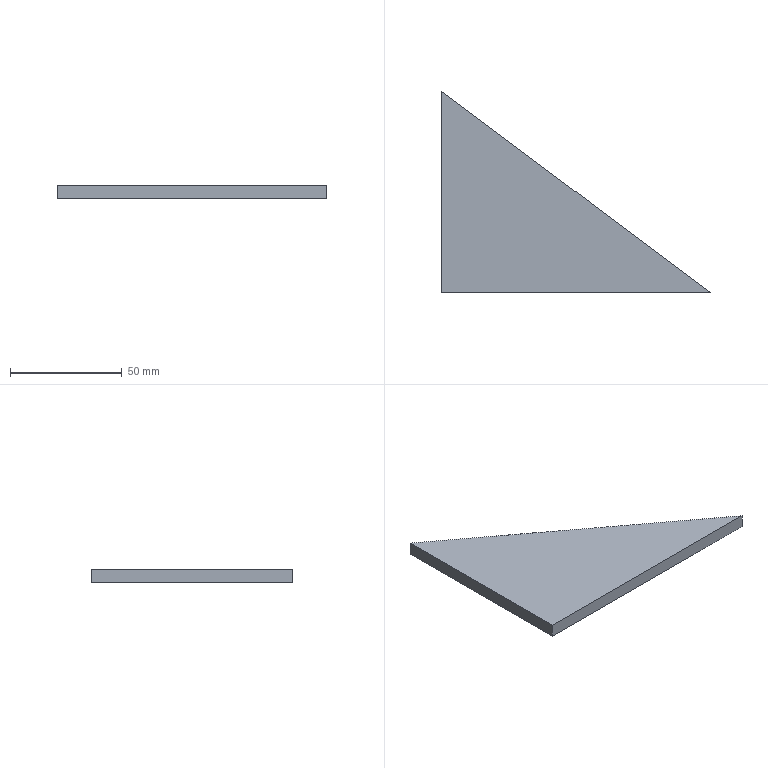Part | STEP file | BCC3 H17_3 | 1 solid | 5 faces | box 120 x 90 x 6 mm | volume 32400 mm3 | plane 5
STEP:
#1=CARTESIAN_POINT('',(0.,0.,0.));
#2=DIRECTION('',(0.,0.,1.));
#3=DIRECTION('',(1.,0.,0.));
#4=AXIS2_PLACEMENT_3D('',#1,#2,#3);
#5=CARTESIAN_POINT('',(0.,0.,0.));
#6=VERTEX_POINT('',#5);
#7=CARTESIAN_POINT('',(120.,0.,0.));
#8=VERTEX_POINT('',#7);
#9=CARTESIAN_POINT('',(120.,0.,0.));
#10=DIRECTION('',(1.,0.,0.));
#11=VECTOR('',#10,1.);
#12=LINE('',#9,#11);
#13=CARTESIAN_POINT('',(120.,0.,6.));
#14=DIRECTION('',(0.,1.,0.));
#15=DIRECTION('',(-1.,0.,0.));
#16=AXIS2_PLACEMENT_3D('',#13,#14,#15);
#17=PLANE('',#16);
#18=CARTESIAN_POINT('',(0.,-6.));
#19=DIRECTION('',(-1.,0.));
#20=VECTOR('',#19,1.);
#21=LINE('',#18,#20);
#22=(GEOMETRIC_REPRESENTATION_CONTEXT(2)PARAMETRIC_REPRESENTATION_CONTEXT()REPRESENTATION_CONTEXT('',''));
#23=DEFINITIONAL_REPRESENTATION('',(#21),#22);
#24=PCURVE('',#17,#23);
#25=CARTESIAN_POINT('',(0.,0.,0.));
#26=DIRECTION('',(0.,0.,-1.));
#27=DIRECTION('',(-1.,0.,0.));
#28=AXIS2_PLACEMENT_3D('',#25,#26,#27);
#29=PLANE('',#28);
#30=CARTESIAN_POINT('',(-120.,0.));
#31=DIRECTION('',(-1.,0.));
#32=VECTOR('',#31,1.);
#33=LINE('',#30,#32);
#34=(GEOMETRIC_REPRESENTATION_CONTEXT(2)PARAMETRIC_REPRESENTATION_CONTEXT()REPRESENTATION_CONTEXT('',''));
#35=DEFINITIONAL_REPRESENTATION('',(#33),#34);
#36=PCURVE('',#29,#35);
#37=SURFACE_CURVE('',#12,(#24,#36),.PCURVE_S1.);
#38=EDGE_CURVE('',#6,#8,#37,.T.);
#39=ORIENTED_EDGE('',*,*,#38,.T.);
#40=CARTESIAN_POINT('',(120.,0.,6.));
#41=VERTEX_POINT('',#40);
#42=CARTESIAN_POINT('',(120.,0.,6.));
#43=DIRECTION('',(0.,0.,-1.));
#44=VECTOR('',#43,1.);
#45=LINE('',#42,#44);
#46=CARTESIAN_POINT('',(0.,0.));
#47=DIRECTION('',(0.,-1.));
#48=VECTOR('',#47,1.);
#49=LINE('',#46,#48);
#50=(GEOMETRIC_REPRESENTATION_CONTEXT(2)PARAMETRIC_REPRESENTATION_CONTEXT()REPRESENTATION_CONTEXT('',''));
#51=DEFINITIONAL_REPRESENTATION('',(#49),#50);
#52=PCURVE('',#17,#51);
#53=CARTESIAN_POINT('',(0.,90.,6.));
#54=DIRECTION('',(-0.6,-0.8,0.));
#55=DIRECTION('',(0.8,-0.6,0.));
#56=AXIS2_PLACEMENT_3D('',#53,#54,#55);
#57=PLANE('',#56);
#58=CARTESIAN_POINT('',(150.,0.));
#59=DIRECTION('',(0.,-1.));
#60=VECTOR('',#59,1.);
#61=LINE('',#58,#60);
#62=(GEOMETRIC_REPRESENTATION_CONTEXT(2)PARAMETRIC_REPRESENTATION_CONTEXT()REPRESENTATION_CONTEXT('',''));
#63=DEFINITIONAL_REPRESENTATION('',(#61),#62);
#64=PCURVE('',#57,#63);
#65=SURFACE_CURVE('',#45,(#52,#64),.PCURVE_S1.);
#66=EDGE_CURVE('',#41,#8,#65,.T.);
#67=ORIENTED_EDGE('',*,*,#66,.F.);
#68=CARTESIAN_POINT('',(0.,0.,6.));
#69=VERTEX_POINT('',#68);
#70=CARTESIAN_POINT('',(120.,0.,6.));
#71=DIRECTION('',(1.,0.,0.));
#72=VECTOR('',#71,1.);
#73=LINE('',#70,#72);
#74=CARTESIAN_POINT('',(0.,0.));
#75=DIRECTION('',(-1.,0.));
#76=VECTOR('',#75,1.);
#77=LINE('',#74,#76);
#78=(GEOMETRIC_REPRESENTATION_CONTEXT(2)PARAMETRIC_REPRESENTATION_CONTEXT()REPRESENTATION_CONTEXT('',''));
#79=DEFINITIONAL_REPRESENTATION('',(#77),#78);
#80=PCURVE('',#17,#79);
#81=CARTESIAN_POINT('',(0.,0.,6.));
#82=DIRECTION('',(0.,0.,-1.));
#83=DIRECTION('',(-1.,0.,0.));
#84=AXIS2_PLACEMENT_3D('',#81,#82,#83);
#85=PLANE('',#84);
#86=CARTESIAN_POINT('',(-120.,0.));
#87=DIRECTION('',(-1.,0.));
#88=VECTOR('',#87,1.);
#89=LINE('',#86,#88);
#90=(GEOMETRIC_REPRESENTATION_CONTEXT(2)PARAMETRIC_REPRESENTATION_CONTEXT()REPRESENTATION_CONTEXT('',''));
#91=DEFINITIONAL_REPRESENTATION('',(#89),#90);
#92=PCURVE('',#85,#91);
#93=SURFACE_CURVE('',#73,(#80,#92),.PCURVE_S1.);
#94=EDGE_CURVE('',#69,#41,#93,.T.);
#95=ORIENTED_EDGE('',*,*,#94,.F.);
#96=CARTESIAN_POINT('',(0.,0.,6.));
#97=DIRECTION('',(0.,0.,-1.));
#98=VECTOR('',#97,1.);
#99=LINE('',#96,#98);
#100=CARTESIAN_POINT('',(120.,0.));
#101=DIRECTION('',(0.,-1.));
#102=VECTOR('',#101,1.);
#103=LINE('',#100,#102);
#104=(GEOMETRIC_REPRESENTATION_CONTEXT(2)PARAMETRIC_REPRESENTATION_CONTEXT()REPRESENTATION_CONTEXT('',''));
#105=DEFINITIONAL_REPRESENTATION('',(#103),#104);
#106=PCURVE('',#17,#105);
#107=CARTESIAN_POINT('',(0.,0.,6.));
#108=DIRECTION('',(1.,0.,0.));
#109=DIRECTION('',(0.,0.,-1.));
#110=AXIS2_PLACEMENT_3D('',#107,#108,#109);
#111=PLANE('',#110);
#112=CARTESIAN_POINT('',(0.,0.));
#113=DIRECTION('',(1.,0.));
#114=VECTOR('',#113,1.);
#115=LINE('',#112,#114);
#116=(GEOMETRIC_REPRESENTATION_CONTEXT(2)PARAMETRIC_REPRESENTATION_CONTEXT()REPRESENTATION_CONTEXT('',''));
#117=DEFINITIONAL_REPRESENTATION('',(#115),#116);
#118=PCURVE('',#111,#117);
#119=SURFACE_CURVE('',#99,(#106,#118),.PCURVE_S1.);
#120=EDGE_CURVE('',#69,#6,#119,.T.);
#121=ORIENTED_EDGE('',*,*,#120,.T.);
#122=EDGE_LOOP('',(#39,#67,#95,#121));
#123=FACE_BOUND('',#122,.T.);
#124=ADVANCED_FACE('',(#123),#17,.F.);
#125=CARTESIAN_POINT('',(0.,90.,0.));
#126=VERTEX_POINT('',#125);
#127=CARTESIAN_POINT('',(0.,90.,0.));
#128=DIRECTION('',(-0.8,0.6,0.));
#129=VECTOR('',#128,1.);
#130=LINE('',#127,#129);
#131=CARTESIAN_POINT('',(0.,-6.));
#132=DIRECTION('',(-1.,0.));
#133=VECTOR('',#132,1.);
#134=LINE('',#131,#133);
#135=(GEOMETRIC_REPRESENTATION_CONTEXT(2)PARAMETRIC_REPRESENTATION_CONTEXT()REPRESENTATION_CONTEXT('',''));
#136=DEFINITIONAL_REPRESENTATION('',(#134),#135);
#137=PCURVE('',#57,#136);
#138=CARTESIAN_POINT('',(0.,90.));
#139=DIRECTION('',(0.8,0.6));
#140=VECTOR('',#139,1.);
#141=LINE('',#138,#140);
#142=(GEOMETRIC_REPRESENTATION_CONTEXT(2)PARAMETRIC_REPRESENTATION_CONTEXT()REPRESENTATION_CONTEXT('',''));
#143=DEFINITIONAL_REPRESENTATION('',(#141),#142);
#144=PCURVE('',#29,#143);
#145=SURFACE_CURVE('',#130,(#137,#144),.PCURVE_S1.);
#146=EDGE_CURVE('',#8,#126,#145,.T.);
#147=ORIENTED_EDGE('',*,*,#146,.T.);
#148=CARTESIAN_POINT('',(0.,90.,6.));
#149=VERTEX_POINT('',#148);
#150=CARTESIAN_POINT('',(0.,90.,6.));
#151=DIRECTION('',(0.,0.,-1.));
#152=VECTOR('',#151,1.);
#153=LINE('',#150,#152);
#154=CARTESIAN_POINT('',(0.,0.));
#155=DIRECTION('',(0.,-1.));
#156=VECTOR('',#155,1.);
#157=LINE('',#154,#156);
#158=(GEOMETRIC_REPRESENTATION_CONTEXT(2)PARAMETRIC_REPRESENTATION_CONTEXT()REPRESENTATION_CONTEXT('',''));
#159=DEFINITIONAL_REPRESENTATION('',(#157),#158);
#160=PCURVE('',#57,#159);
#161=CARTESIAN_POINT('',(0.,90.));
#162=DIRECTION('',(1.,0.));
#163=VECTOR('',#162,1.);
#164=LINE('',#161,#163);
#165=(GEOMETRIC_REPRESENTATION_CONTEXT(2)PARAMETRIC_REPRESENTATION_CONTEXT()REPRESENTATION_CONTEXT('',''));
#166=DEFINITIONAL_REPRESENTATION('',(#164),#165);
#167=PCURVE('',#111,#166);
#168=SURFACE_CURVE('',#153,(#160,#167),.PCURVE_S1.);
#169=EDGE_CURVE('',#149,#126,#168,.T.);
#170=ORIENTED_EDGE('',*,*,#169,.F.);
#171=CARTESIAN_POINT('',(0.,90.,6.));
#172=DIRECTION('',(-0.8,0.6,0.));
#173=VECTOR('',#172,1.);
#174=LINE('',#171,#173);
#175=CARTESIAN_POINT('',(0.,0.));
#176=DIRECTION('',(-1.,0.));
#177=VECTOR('',#176,1.);
#178=LINE('',#175,#177);
#179=(GEOMETRIC_REPRESENTATION_CONTEXT(2)PARAMETRIC_REPRESENTATION_CONTEXT()REPRESENTATION_CONTEXT('',''));
#180=DEFINITIONAL_REPRESENTATION('',(#178),#179);
#181=PCURVE('',#57,#180);
#182=CARTESIAN_POINT('',(0.,90.));
#183=DIRECTION('',(0.8,0.6));
#184=VECTOR('',#183,1.);
#185=LINE('',#182,#184);
#186=(GEOMETRIC_REPRESENTATION_CONTEXT(2)PARAMETRIC_REPRESENTATION_CONTEXT()REPRESENTATION_CONTEXT('',''));
#187=DEFINITIONAL_REPRESENTATION('',(#185),#186);
#188=PCURVE('',#85,#187);
#189=SURFACE_CURVE('',#174,(#181,#188),.PCURVE_S1.);
#190=EDGE_CURVE('',#41,#149,#189,.T.);
#191=ORIENTED_EDGE('',*,*,#190,.F.);
#192=ORIENTED_EDGE('',*,*,#66,.T.);
#193=EDGE_LOOP('',(#147,#170,#191,#192));
#194=FACE_BOUND('',#193,.T.);
#195=ADVANCED_FACE('',(#194),#57,.F.);
#196=CARTESIAN_POINT('',(0.,0.,0.));
#197=DIRECTION('',(0.,-1.,0.));
#198=VECTOR('',#197,1.);
#199=LINE('',#196,#198);
#200=CARTESIAN_POINT('',(6.,0.));
#201=DIRECTION('',(0.,-1.));
#202=VECTOR('',#201,1.);
#203=LINE('',#200,#202);
#204=(GEOMETRIC_REPRESENTATION_CONTEXT(2)PARAMETRIC_REPRESENTATION_CONTEXT()REPRESENTATION_CONTEXT('',''));
#205=DEFINITIONAL_REPRESENTATION('',(#203),#204);
#206=PCURVE('',#111,#205);
#207=CARTESIAN_POINT('',(0.,0.));
#208=DIRECTION('',(0.,-1.));
#209=VECTOR('',#208,1.);
#210=LINE('',#207,#209);
#211=(GEOMETRIC_REPRESENTATION_CONTEXT(2)PARAMETRIC_REPRESENTATION_CONTEXT()REPRESENTATION_CONTEXT('',''));
#212=DEFINITIONAL_REPRESENTATION('',(#210),#211);
#213=PCURVE('',#29,#212);
#214=SURFACE_CURVE('',#199,(#206,#213),.PCURVE_S1.);
#215=EDGE_CURVE('',#126,#6,#214,.T.);
#216=ORIENTED_EDGE('',*,*,#215,.T.);
#217=ORIENTED_EDGE('',*,*,#120,.F.);
#218=CARTESIAN_POINT('',(0.,0.,6.));
#219=DIRECTION('',(0.,-1.,0.));
#220=VECTOR('',#219,1.);
#221=LINE('',#218,#220);
#222=CARTESIAN_POINT('',(0.,0.));
#223=DIRECTION('',(0.,-1.));
#224=VECTOR('',#223,1.);
#225=LINE('',#222,#224);
#226=(GEOMETRIC_REPRESENTATION_CONTEXT(2)PARAMETRIC_REPRESENTATION_CONTEXT()REPRESENTATION_CONTEXT('',''));
#227=DEFINITIONAL_REPRESENTATION('',(#225),#226);
#228=PCURVE('',#111,#227);
#229=CARTESIAN_POINT('',(0.,0.));
#230=DIRECTION('',(0.,-1.));
#231=VECTOR('',#230,1.);
#232=LINE('',#229,#231);
#233=(GEOMETRIC_REPRESENTATION_CONTEXT(2)PARAMETRIC_REPRESENTATION_CONTEXT()REPRESENTATION_CONTEXT('',''));
#234=DEFINITIONAL_REPRESENTATION('',(#232),#233);
#235=PCURVE('',#85,#234);
#236=SURFACE_CURVE('',#221,(#228,#235),.PCURVE_S1.);
#237=EDGE_CURVE('',#149,#69,#236,.T.);
#238=ORIENTED_EDGE('',*,*,#237,.F.);
#239=ORIENTED_EDGE('',*,*,#169,.T.);
#240=EDGE_LOOP('',(#216,#217,#238,#239));
#241=FACE_BOUND('',#240,.T.);
#242=ADVANCED_FACE('',(#241),#111,.F.);
#243=ORIENTED_EDGE('',*,*,#94,.T.);
#244=ORIENTED_EDGE('',*,*,#190,.T.);
#245=ORIENTED_EDGE('',*,*,#237,.T.);
#246=EDGE_LOOP('',(#243,#244,#245));
#247=FACE_BOUND('',#246,.T.);
#248=ADVANCED_FACE('',(#247),#85,.F.);
#249=ORIENTED_EDGE('',*,*,#38,.F.);
#250=ORIENTED_EDGE('',*,*,#215,.F.);
#251=ORIENTED_EDGE('',*,*,#146,.F.);
#252=EDGE_LOOP('',(#249,#250,#251));
#253=FACE_BOUND('',#252,.T.);
#254=ADVANCED_FACE('',(#253),#29,.T.);
#255=CLOSED_SHELL('',(#124,#195,#242,#248,#254));
#256=MANIFOLD_SOLID_BREP('',#255);
#257=(LENGTH_UNIT()NAMED_UNIT(*)SI_UNIT(.MILLI.,.METRE.));
#258=UNCERTAINTY_MEASURE_WITH_UNIT(LENGTH_MEASURE(0.0000001),#257,'','');
#259=(NAMED_UNIT(*)PLANE_ANGLE_UNIT()SI_UNIT($,.RADIAN.));
#260=(NAMED_UNIT(*)SI_UNIT($,.STERADIAN.)SOLID_ANGLE_UNIT());
#261=(GEOMETRIC_REPRESENTATION_CONTEXT(3)GLOBAL_UNCERTAINTY_ASSIGNED_CONTEXT((#258))GLOBAL_UNIT_ASSIGNED_CONTEXT((#257,#259,#260))REPRESENTATION_CONTEXT('',''));
#262=ADVANCED_BREP_SHAPE_REPRESENTATION('',(#4,#256),#261);